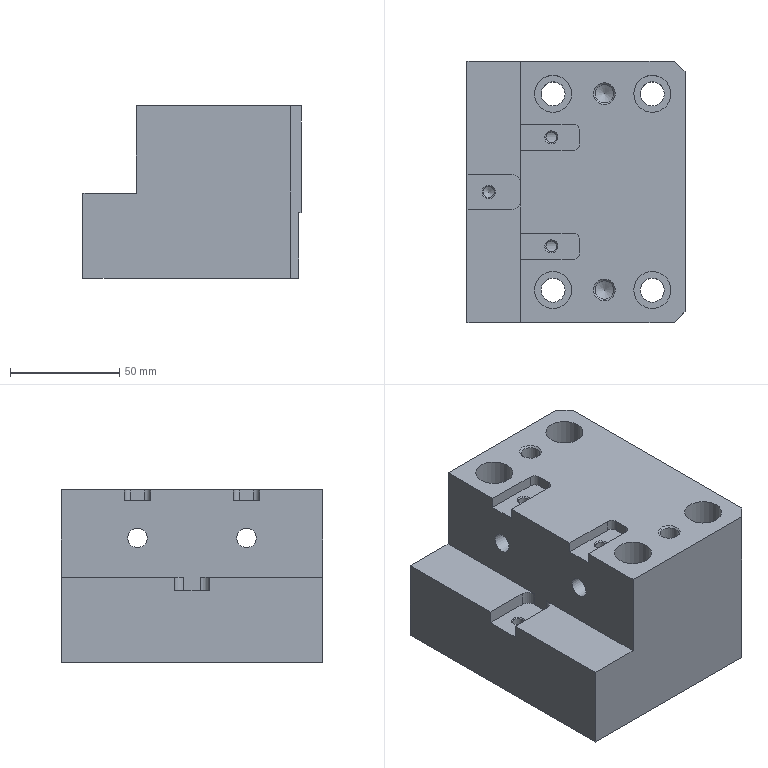Part | STEP file | gslz 2016.10.28-6_id694_x_t | 1 solid | 70 faces | box 100 x 120 x 79 mm | volume 734438 mm3 | plane 36 | cylinder 26 | cone 8 | commonest cylinder face diameters 6 x4 11 x4 17 x4 5 x3 8 x2 8.5 x2